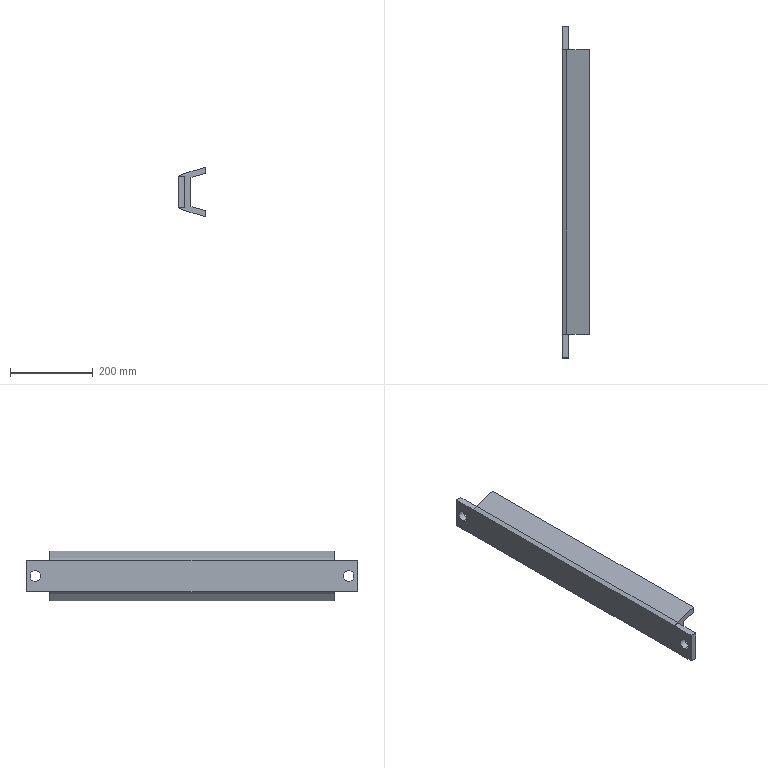Part | SolidWorks | features ICE 2, Extrusion 1, MirrorPattern 1 | 1 solid | 24 faces | box 65 x 800 x 120 mm | volume 2622134 mm3 | plane 20 | cylinder 4 | commonest cylinder face diameters 26 x4
STEP:
#1=CARTESIAN_POINT('',(15.,-377.5,-13.));
#2=VERTEX_POINT('',#1);
#3=CARTESIAN_POINT('',(15.,-377.5,13.));
#4=VERTEX_POINT('',#3);
#5=CARTESIAN_POINT('',(15.,-377.5,0.));
#6=DIRECTION('',(-1.,0.,0.));
#7=DIRECTION('',(0.,0.,1.));
#8=AXIS2_PLACEMENT_3D('',#5,#6,#7);
#9=CIRCLE('',#8,13.);
#10=EDGE_CURVE('',#2,#4,#9,.T.);
#11=ORIENTED_EDGE('',*,*,#10,.F.);
#12=CARTESIAN_POINT('',(0.,-377.5,-13.));
#13=VERTEX_POINT('',#12);
#14=CARTESIAN_POINT('',(57.5,-377.5,-13.));
#15=DIRECTION('',(-1.,0.,0.));
#16=VECTOR('',#15,1000.);
#17=LINE('',#14,#16);
#18=EDGE_CURVE('',#2,#13,#17,.T.);
#19=ORIENTED_EDGE('',*,*,#18,.T.);
#20=CARTESIAN_POINT('',(0.,-377.5,13.));
#21=VERTEX_POINT('',#20);
#22=CARTESIAN_POINT('',(0.,-377.5,0.));
#23=DIRECTION('',(-1.,0.,0.));
#24=DIRECTION('',(0.,0.,1.));
#25=AXIS2_PLACEMENT_3D('',#22,#23,#24);
#26=CIRCLE('',#25,13.);
#27=EDGE_CURVE('',#13,#21,#26,.T.);
#28=ORIENTED_EDGE('',*,*,#27,.T.);
#29=CARTESIAN_POINT('',(57.5,-377.5,13.));
#30=DIRECTION('',(-1.,0.,0.));
#31=VECTOR('',#30,1000.);
#32=LINE('',#29,#31);
#33=EDGE_CURVE('',#4,#21,#32,.T.);
#34=ORIENTED_EDGE('',*,*,#33,.F.);
#35=EDGE_LOOP('',(#11,#19,#28,#34));
#36=FACE_OUTER_BOUND('',#35,.T.);
#37=CARTESIAN_POINT('',(57.5,-377.5,0.));
#38=DIRECTION('',(-1.,0.,0.));
#39=DIRECTION('',(0.,0.,1.));
#40=AXIS2_PLACEMENT_3D('',#37,#38,#39);
#41=CYLINDRICAL_SURFACE('',#40,13.);
#42=ADVANCED_FACE('',(#36),#41,.F.);
#43=CARTESIAN_POINT('',(15.,377.5,13.));
#44=VERTEX_POINT('',#43);
#45=CARTESIAN_POINT('',(15.,377.5,-13.));
#46=VERTEX_POINT('',#45);
#47=CARTESIAN_POINT('',(15.,377.5,0.));
#48=DIRECTION('',(1.,0.,0.));
#49=DIRECTION('',(0.,0.,-1.));
#50=AXIS2_PLACEMENT_3D('',#47,#48,#49);
#51=CIRCLE('',#50,13.);
#52=EDGE_CURVE('',#44,#46,#51,.T.);
#53=ORIENTED_EDGE('',*,*,#52,.T.);
#54=CARTESIAN_POINT('',(0.,377.5,-13.));
#55=VERTEX_POINT('',#54);
#56=CARTESIAN_POINT('',(57.5,377.5,-13.));
#57=DIRECTION('',(-1.,0.,0.));
#58=VECTOR('',#57,1000.);
#59=LINE('',#56,#58);
#60=EDGE_CURVE('',#46,#55,#59,.T.);
#61=ORIENTED_EDGE('',*,*,#60,.T.);
#62=CARTESIAN_POINT('',(0.,377.5,13.));
#63=VERTEX_POINT('',#62);
#64=CARTESIAN_POINT('',(0.,377.5,0.));
#65=DIRECTION('',(-1.,0.,0.));
#66=DIRECTION('',(0.,0.,1.));
#67=AXIS2_PLACEMENT_3D('',#64,#65,#66);
#68=CIRCLE('',#67,13.);
#69=EDGE_CURVE('',#55,#63,#68,.T.);
#70=ORIENTED_EDGE('',*,*,#69,.T.);
#71=CARTESIAN_POINT('',(57.5,377.5,13.));
#72=DIRECTION('',(-1.,0.,0.));
#73=VECTOR('',#72,1000.);
#74=LINE('',#71,#73);
#75=EDGE_CURVE('',#44,#63,#74,.T.);
#76=ORIENTED_EDGE('',*,*,#75,.F.);
#77=EDGE_LOOP('',(#53,#61,#70,#76));
#78=FACE_OUTER_BOUND('',#77,.T.);
#79=CARTESIAN_POINT('',(57.5,377.5,0.));
#80=DIRECTION('',(-1.,0.,0.));
#81=DIRECTION('',(0.,0.,1.));
#82=AXIS2_PLACEMENT_3D('',#79,#80,#81);
#83=CYLINDRICAL_SURFACE('',#82,13.);
#84=ADVANCED_FACE('',(#78),#83,.F.);
#85=CARTESIAN_POINT('',(10.,342.5,-42.882));
#86=VERTEX_POINT('',#85);
#87=CARTESIAN_POINT('',(0.,342.5,-37.5));
#88=VERTEX_POINT('',#87);
#89=CARTESIAN_POINT('',(0.,342.5,-37.5));
#90=DIRECTION('',(-0.8806,0.,0.4739));
#91=VECTOR('',#90,1000.);
#92=LINE('',#89,#91);
#93=EDGE_CURVE('',#86,#88,#92,.T.);
#94=ORIENTED_EDGE('',*,*,#93,.T.);
#95=CARTESIAN_POINT('',(15.,342.5,-37.5));
#96=VERTEX_POINT('',#95);
#97=CARTESIAN_POINT('',(0.,342.5,-37.5));
#98=DIRECTION('',(1.,0.,0.));
#99=VECTOR('',#98,1000.);
#100=LINE('',#97,#99);
#101=EDGE_CURVE('',#88,#96,#100,.T.);
#102=ORIENTED_EDGE('',*,*,#101,.T.);
#103=CARTESIAN_POINT('',(15.,342.5,37.5));
#104=VERTEX_POINT('',#103);
#105=CARTESIAN_POINT('',(15.,342.5,37.5));
#106=DIRECTION('',(0.,0.,1.));
#107=VECTOR('',#106,1000.);
#108=LINE('',#105,#107);
#109=EDGE_CURVE('',#96,#104,#108,.T.);
#110=ORIENTED_EDGE('',*,*,#109,.T.);
#111=CARTESIAN_POINT('',(0.,342.5,37.5));
#112=VERTEX_POINT('',#111);
#113=CARTESIAN_POINT('',(0.,342.5,37.5));
#114=DIRECTION('',(-1.,0.,0.));
#115=VECTOR('',#114,1000.);
#116=LINE('',#113,#115);
#117=EDGE_CURVE('',#104,#112,#116,.T.);
#118=ORIENTED_EDGE('',*,*,#117,.T.);
#119=CARTESIAN_POINT('',(10.,342.5,42.882));
#120=VERTEX_POINT('',#119);
#121=CARTESIAN_POINT('',(0.,342.5,37.5));
#122=DIRECTION('',(0.8806,0.,0.4739));
#123=VECTOR('',#122,1000.);
#124=LINE('',#121,#123);
#125=EDGE_CURVE('',#112,#120,#124,.T.);
#126=ORIENTED_EDGE('',*,*,#125,.T.);
#127=CARTESIAN_POINT('',(65.,342.5,60.));
#128=VERTEX_POINT('',#127);
#129=CARTESIAN_POINT('',(10.,342.5,42.882));
#130=DIRECTION('',(0.9548,0.,0.2972));
#131=VECTOR('',#130,1000.);
#132=LINE('',#129,#131);
#133=EDGE_CURVE('',#120,#128,#132,.T.);
#134=ORIENTED_EDGE('',*,*,#133,.T.);
#135=CARTESIAN_POINT('',(65.,342.5,45.));
#136=VERTEX_POINT('',#135);
#137=CARTESIAN_POINT('',(65.,342.5,60.));
#138=DIRECTION('',(0.,0.,-1.));
#139=VECTOR('',#138,1000.);
#140=LINE('',#137,#139);
#141=EDGE_CURVE('',#128,#136,#140,.T.);
#142=ORIENTED_EDGE('',*,*,#141,.T.);
#143=CARTESIAN_POINT('',(30.,342.5,35.));
#144=VERTEX_POINT('',#143);
#145=CARTESIAN_POINT('',(65.,342.5,45.));
#146=DIRECTION('',(-0.9615,0.,-0.2747));
#147=VECTOR('',#146,1000.);
#148=LINE('',#145,#147);
#149=EDGE_CURVE('',#136,#144,#148,.T.);
#150=ORIENTED_EDGE('',*,*,#149,.T.);
#151=CARTESIAN_POINT('',(30.,342.5,-35.));
#152=VERTEX_POINT('',#151);
#153=CARTESIAN_POINT('',(30.,342.5,-35.));
#154=DIRECTION('',(0.,0.,-1.));
#155=VECTOR('',#154,1000.);
#156=LINE('',#153,#155);
#157=EDGE_CURVE('',#144,#152,#156,.T.);
#158=ORIENTED_EDGE('',*,*,#157,.T.);
#159=CARTESIAN_POINT('',(65.,342.5,-45.));
#160=VERTEX_POINT('',#159);
#161=CARTESIAN_POINT('',(65.,342.5,-45.));
#162=DIRECTION('',(0.9615,0.,-0.2747));
#163=VECTOR('',#162,1000.);
#164=LINE('',#161,#163);
#165=EDGE_CURVE('',#152,#160,#164,.T.);
#166=ORIENTED_EDGE('',*,*,#165,.T.);
#167=CARTESIAN_POINT('',(65.,342.5,-60.));
#168=VERTEX_POINT('',#167);
#169=CARTESIAN_POINT('',(65.,342.5,-60.));
#170=DIRECTION('',(0.,0.,-1.));
#171=VECTOR('',#170,1000.);
#172=LINE('',#169,#171);
#173=EDGE_CURVE('',#160,#168,#172,.T.);
#174=ORIENTED_EDGE('',*,*,#173,.T.);
#175=CARTESIAN_POINT('',(10.,342.5,-42.882));
#176=DIRECTION('',(-0.9548,0.,0.2972));
#177=VECTOR('',#176,1000.);
#178=LINE('',#175,#177);
#179=EDGE_CURVE('',#168,#86,#178,.T.);
#180=ORIENTED_EDGE('',*,*,#179,.T.);
#181=EDGE_LOOP('',(#94,#102,#110,#118,#126,#134,#142,#150,#158,#166,#174,#180));
#182=FACE_OUTER_BOUND('',#181,.T.);
#183=CARTESIAN_POINT('',(0.,342.5,0.));
#184=DIRECTION('',(0.,1.,0.));
#185=DIRECTION('',(0.,0.,1.));
#186=AXIS2_PLACEMENT_3D('',#183,#184,#185);
#187=PLANE('',#186);
#188=ADVANCED_FACE('',(#182),#187,.T.);
#189=CARTESIAN_POINT('',(15.,-342.5,37.5));
#190=VERTEX_POINT('',#189);
#191=CARTESIAN_POINT('',(0.,-342.5,37.5));
#192=VERTEX_POINT('',#191);
#193=CARTESIAN_POINT('',(0.,-342.5,37.5));
#194=DIRECTION('',(-1.,0.,0.));
#195=VECTOR('',#194,1000.);
#196=LINE('',#193,#195);
#197=EDGE_CURVE('',#190,#192,#196,.T.);
#198=ORIENTED_EDGE('',*,*,#197,.F.);
#199=CARTESIAN_POINT('',(15.,-342.5,-37.5));
#200=VERTEX_POINT('',#199);
#201=CARTESIAN_POINT('',(15.,-342.5,37.5));
#202=DIRECTION('',(0.,0.,1.));
#203=VECTOR('',#202,1000.);
#204=LINE('',#201,#203);
#205=EDGE_CURVE('',#200,#190,#204,.T.);
#206=ORIENTED_EDGE('',*,*,#205,.F.);
#207=CARTESIAN_POINT('',(0.,-342.5,-37.5));
#208=VERTEX_POINT('',#207);
#209=CARTESIAN_POINT('',(0.,-342.5,-37.5));
#210=DIRECTION('',(1.,0.,0.));
#211=VECTOR('',#210,1000.);
#212=LINE('',#209,#211);
#213=EDGE_CURVE('',#208,#200,#212,.T.);
#214=ORIENTED_EDGE('',*,*,#213,.F.);
#215=CARTESIAN_POINT('',(10.,-342.5,-42.882));
#216=VERTEX_POINT('',#215);
#217=CARTESIAN_POINT('',(0.,-342.5,-37.5));
#218=DIRECTION('',(-0.8806,0.,0.4739));
#219=VECTOR('',#218,1000.);
#220=LINE('',#217,#219);
#221=EDGE_CURVE('',#216,#208,#220,.T.);
#222=ORIENTED_EDGE('',*,*,#221,.F.);
#223=CARTESIAN_POINT('',(65.,-342.5,-60.));
#224=VERTEX_POINT('',#223);
#225=CARTESIAN_POINT('',(10.,-342.5,-42.882));
#226=DIRECTION('',(-0.9548,0.,0.2972));
#227=VECTOR('',#226,1000.);
#228=LINE('',#225,#227);
#229=EDGE_CURVE('',#224,#216,#228,.T.);
#230=ORIENTED_EDGE('',*,*,#229,.F.);
#231=CARTESIAN_POINT('',(65.,-342.5,-45.));
#232=VERTEX_POINT('',#231);
#233=CARTESIAN_POINT('',(65.,-342.5,-60.));
#234=DIRECTION('',(0.,0.,-1.));
#235=VECTOR('',#234,1000.);
#236=LINE('',#233,#235);
#237=EDGE_CURVE('',#232,#224,#236,.T.);
#238=ORIENTED_EDGE('',*,*,#237,.F.);
#239=CARTESIAN_POINT('',(30.,-342.5,-35.));
#240=VERTEX_POINT('',#239);
#241=CARTESIAN_POINT('',(65.,-342.5,-45.));
#242=DIRECTION('',(0.9615,0.,-0.2747));
#243=VECTOR('',#242,1000.);
#244=LINE('',#241,#243);
#245=EDGE_CURVE('',#240,#232,#244,.T.);
#246=ORIENTED_EDGE('',*,*,#245,.F.);
#247=CARTESIAN_POINT('',(30.,-342.5,35.));
#248=VERTEX_POINT('',#247);
#249=CARTESIAN_POINT('',(30.,-342.5,-35.));
#250=DIRECTION('',(0.,0.,-1.));
#251=VECTOR('',#250,1000.);
#252=LINE('',#249,#251);
#253=EDGE_CURVE('',#248,#240,#252,.T.);
#254=ORIENTED_EDGE('',*,*,#253,.F.);
#255=CARTESIAN_POINT('',(65.,-342.5,45.));
#256=VERTEX_POINT('',#255);
#257=CARTESIAN_POINT('',(65.,-342.5,45.));
#258=DIRECTION('',(-0.9615,0.,-0.2747));
#259=VECTOR('',#258,1000.);
#260=LINE('',#257,#259);
#261=EDGE_CURVE('',#256,#248,#260,.T.);
#262=ORIENTED_EDGE('',*,*,#261,.F.);
#263=CARTESIAN_POINT('',(65.,-342.5,60.));
#264=VERTEX_POINT('',#263);
#265=CARTESIAN_POINT('',(65.,-342.5,60.));
#266=DIRECTION('',(0.,0.,-1.));
#267=VECTOR('',#266,1000.);
#268=LINE('',#265,#267);
#269=EDGE_CURVE('',#264,#256,#268,.T.);
#270=ORIENTED_EDGE('',*,*,#269,.F.);
#271=CARTESIAN_POINT('',(10.,-342.5,42.882));
#272=VERTEX_POINT('',#271);
#273=CARTESIAN_POINT('',(10.,-342.5,42.882));
#274=DIRECTION('',(0.9548,0.,0.2972));
#275=VECTOR('',#274,1000.);
#276=LINE('',#273,#275);
#277=EDGE_CURVE('',#272,#264,#276,.T.);
#278=ORIENTED_EDGE('',*,*,#277,.F.);
#279=CARTESIAN_POINT('',(0.,-342.5,37.5));
#280=DIRECTION('',(0.8806,0.,0.4739));
#281=VECTOR('',#280,1000.);
#282=LINE('',#279,#281);
#283=EDGE_CURVE('',#192,#272,#282,.T.);
#284=ORIENTED_EDGE('',*,*,#283,.F.);
#285=EDGE_LOOP('',(#198,#206,#214,#222,#230,#238,#246,#254,#262,#270,#278,#284));
#286=FACE_OUTER_BOUND('',#285,.T.);
#287=CARTESIAN_POINT('',(0.,-342.5,0.));
#288=DIRECTION('',(0.,1.,0.));
#289=DIRECTION('',(0.,0.,1.));
#290=AXIS2_PLACEMENT_3D('',#287,#288,#289);
#291=PLANE('',#290);
#292=ADVANCED_FACE('',(#286),#291,.F.);
#293=ORIENTED_EDGE('',*,*,#261,.T.);
#294=CARTESIAN_POINT('',(30.,342.5,35.));
#295=DIRECTION('',(0.,-1.,0.));
#296=VECTOR('',#295,1000.);
#297=LINE('',#294,#296);
#298=EDGE_CURVE('',#144,#248,#297,.T.);
#299=ORIENTED_EDGE('',*,*,#298,.F.);
#300=ORIENTED_EDGE('',*,*,#149,.F.);
#301=CARTESIAN_POINT('',(65.,342.5,45.));
#302=DIRECTION('',(0.,-1.,0.));
#303=VECTOR('',#302,1000.);
#304=LINE('',#301,#303);
#305=EDGE_CURVE('',#136,#256,#304,.T.);
#306=ORIENTED_EDGE('',*,*,#305,.T.);
#307=EDGE_LOOP('',(#293,#299,#300,#306));
#308=FACE_OUTER_BOUND('',#307,.T.);
#309=CARTESIAN_POINT('',(65.,342.5,45.));
#310=DIRECTION('',(-0.2747,0.,0.9615));
#311=DIRECTION('',(0.9615,0.,0.2747));
#312=AXIS2_PLACEMENT_3D('',#309,#310,#311);
#313=PLANE('',#312);
#314=ADVANCED_FACE('',(#308),#313,.F.);
#315=ORIENTED_EDGE('',*,*,#253,.T.);
#316=CARTESIAN_POINT('',(30.,342.5,-35.));
#317=DIRECTION('',(0.,-1.,0.));
#318=VECTOR('',#317,1000.);
#319=LINE('',#316,#318);
#320=EDGE_CURVE('',#152,#240,#319,.T.);
#321=ORIENTED_EDGE('',*,*,#320,.F.);
#322=ORIENTED_EDGE('',*,*,#157,.F.);
#323=ORIENTED_EDGE('',*,*,#298,.T.);
#324=EDGE_LOOP('',(#315,#321,#322,#323));
#325=FACE_OUTER_BOUND('',#324,.T.);
#326=CARTESIAN_POINT('',(30.,342.5,-35.));
#327=DIRECTION('',(-1.,0.,0.));
#328=DIRECTION('',(0.,0.,1.));
#329=AXIS2_PLACEMENT_3D('',#326,#327,#328);
#330=PLANE('',#329);
#331=ADVANCED_FACE('',(#325),#330,.F.);
#332=ORIENTED_EDGE('',*,*,#245,.T.);
#333=CARTESIAN_POINT('',(65.,342.5,-45.));
#334=DIRECTION('',(0.,-1.,0.));
#335=VECTOR('',#334,1000.);
#336=LINE('',#333,#335);
#337=EDGE_CURVE('',#160,#232,#336,.T.);
#338=ORIENTED_EDGE('',*,*,#337,.F.);
#339=ORIENTED_EDGE('',*,*,#165,.F.);
#340=ORIENTED_EDGE('',*,*,#320,.T.);
#341=EDGE_LOOP('',(#332,#338,#339,#340));
#342=FACE_OUTER_BOUND('',#341,.T.);
#343=CARTESIAN_POINT('',(65.,342.5,-45.));
#344=DIRECTION('',(-0.2747,0.,-0.9615));
#345=DIRECTION('',(-0.9615,0.,0.2747));
#346=AXIS2_PLACEMENT_3D('',#343,#344,#345);
#347=PLANE('',#346);
#348=ADVANCED_FACE('',(#342),#347,.F.);
#349=ORIENTED_EDGE('',*,*,#237,.T.);
#350=CARTESIAN_POINT('',(65.,342.5,-60.));
#351=DIRECTION('',(0.,-1.,0.));
#352=VECTOR('',#351,1000.);
#353=LINE('',#350,#352);
#354=EDGE_CURVE('',#168,#224,#353,.T.);
#355=ORIENTED_EDGE('',*,*,#354,.F.);
#356=ORIENTED_EDGE('',*,*,#173,.F.);
#357=ORIENTED_EDGE('',*,*,#337,.T.);
#358=EDGE_LOOP('',(#349,#355,#356,#357));
#359=FACE_OUTER_BOUND('',#358,.T.);
#360=CARTESIAN_POINT('',(65.,342.5,-60.));
#361=DIRECTION('',(-1.,0.,0.));
#362=DIRECTION('',(0.,0.,1.));
#363=AXIS2_PLACEMENT_3D('',#360,#361,#362);
#364=PLANE('',#363);
#365=ADVANCED_FACE('',(#359),#364,.F.);
#366=ORIENTED_EDGE('',*,*,#229,.T.);
#367=CARTESIAN_POINT('',(10.,342.5,-42.882));
#368=DIRECTION('',(0.,-1.,0.));
#369=VECTOR('',#368,1000.);
#370=LINE('',#367,#369);
#371=EDGE_CURVE('',#86,#216,#370,.T.);
#372=ORIENTED_EDGE('',*,*,#371,.F.);
#373=ORIENTED_EDGE('',*,*,#179,.F.);
#374=ORIENTED_EDGE('',*,*,#354,.T.);
#375=EDGE_LOOP('',(#366,#372,#373,#374));
#376=FACE_OUTER_BOUND('',#375,.T.);
#377=CARTESIAN_POINT('',(10.,342.5,-42.882));
#378=DIRECTION('',(0.2972,0.,0.9548));
#379=DIRECTION('',(0.9548,0.,-0.2972));
#380=AXIS2_PLACEMENT_3D('',#377,#378,#379);
#381=PLANE('',#380);
#382=ADVANCED_FACE('',(#376),#381,.F.);
#383=ORIENTED_EDGE('',*,*,#221,.T.);
#384=CARTESIAN_POINT('',(0.,342.5,-37.5));
#385=DIRECTION('',(0.,-1.,0.));
#386=VECTOR('',#385,1000.);
#387=LINE('',#384,#386);
#388=EDGE_CURVE('',#88,#208,#387,.T.);
#389=ORIENTED_EDGE('',*,*,#388,.F.);
#390=ORIENTED_EDGE('',*,*,#93,.F.);
#391=ORIENTED_EDGE('',*,*,#371,.T.);
#392=EDGE_LOOP('',(#383,#389,#390,#391));
#393=FACE_OUTER_BOUND('',#392,.T.);
#394=CARTESIAN_POINT('',(0.,342.5,-37.5));
#395=DIRECTION('',(0.4739,0.,0.8806));
#396=DIRECTION('',(0.8806,0.,-0.4739));
#397=AXIS2_PLACEMENT_3D('',#394,#395,#396);
#398=PLANE('',#397);
#399=ADVANCED_FACE('',(#393),#398,.F.);
#400=CARTESIAN_POINT('',(0.,-377.5,0.));
#401=DIRECTION('',(-1.,0.,0.));
#402=DIRECTION('',(0.,0.,1.));
#403=AXIS2_PLACEMENT_3D('',#400,#401,#402);
#404=CIRCLE('',#403,13.);
#405=EDGE_CURVE('',#21,#13,#404,.T.);
#406=ORIENTED_EDGE('',*,*,#405,.F.);
#407=ORIENTED_EDGE('',*,*,#27,.F.);
#408=EDGE_LOOP('',(#406,#407));
#409=FACE_BOUND('',#408,.T.);
#410=CARTESIAN_POINT('',(0.,377.5,0.));
#411=DIRECTION('',(-1.,0.,0.));
#412=DIRECTION('',(0.,0.,1.));
#413=AXIS2_PLACEMENT_3D('',#410,#411,#412);
#414=CIRCLE('',#413,13.);
#415=EDGE_CURVE('',#63,#55,#414,.T.);
#416=ORIENTED_EDGE('',*,*,#415,.F.);
#417=ORIENTED_EDGE('',*,*,#69,.F.);
#418=EDGE_LOOP('',(#416,#417));
#419=FACE_BOUND('',#418,.T.);
#420=ORIENTED_EDGE('',*,*,#388,.T.);
#421=CARTESIAN_POINT('',(0.,-400.,-37.5));
#422=VERTEX_POINT('',#421);
#423=CARTESIAN_POINT('',(0.,-400.,-37.5));
#424=DIRECTION('',(0.,1.,0.));
#425=VECTOR('',#424,1000.);
#426=LINE('',#423,#425);
#427=EDGE_CURVE('',#422,#208,#426,.T.);
#428=ORIENTED_EDGE('',*,*,#427,.F.);
#429=CARTESIAN_POINT('',(0.,-400.,37.5));
#430=VERTEX_POINT('',#429);
#431=CARTESIAN_POINT('',(0.,-400.,37.5));
#432=DIRECTION('',(0.,0.,-1.));
#433=VECTOR('',#432,1000.);
#434=LINE('',#431,#433);
#435=EDGE_CURVE('',#430,#422,#434,.T.);
#436=ORIENTED_EDGE('',*,*,#435,.F.);
#437=CARTESIAN_POINT('',(0.,-400.,37.5));
#438=DIRECTION('',(0.,1.,0.));
#439=VECTOR('',#438,1000.);
#440=LINE('',#437,#439);
#441=EDGE_CURVE('',#430,#192,#440,.T.);
#442=ORIENTED_EDGE('',*,*,#441,.T.);
#443=CARTESIAN_POINT('',(0.,342.5,37.5));
#444=DIRECTION('',(0.,-1.,0.));
#445=VECTOR('',#444,1000.);
#446=LINE('',#443,#445);
#447=EDGE_CURVE('',#112,#192,#446,.T.);
#448=ORIENTED_EDGE('',*,*,#447,.F.);
#449=CARTESIAN_POINT('',(0.,400.,37.5));
#450=VERTEX_POINT('',#449);
#451=CARTESIAN_POINT('',(0.,400.,37.5));
#452=DIRECTION('',(0.,-1.,0.));
#453=VECTOR('',#452,1000.);
#454=LINE('',#451,#453);
#455=EDGE_CURVE('',#450,#112,#454,.T.);
#456=ORIENTED_EDGE('',*,*,#455,.F.);
#457=CARTESIAN_POINT('',(0.,400.,-37.5));
#458=VERTEX_POINT('',#457);
#459=CARTESIAN_POINT('',(0.,400.,37.5));
#460=DIRECTION('',(0.,0.,-1.));
#461=VECTOR('',#460,1000.);
#462=LINE('',#459,#461);
#463=EDGE_CURVE('',#450,#458,#462,.T.);
#464=ORIENTED_EDGE('',*,*,#463,.T.);
#465=CARTESIAN_POINT('',(0.,400.,-37.5));
#466=DIRECTION('',(0.,-1.,0.));
#467=VECTOR('',#466,1000.);
#468=LINE('',#465,#467);
#469=EDGE_CURVE('',#458,#88,#468,.T.);
#470=ORIENTED_EDGE('',*,*,#469,.T.);
#471=EDGE_LOOP('',(#420,#428,#436,#442,#448,#456,#464,#470));
#472=FACE_OUTER_BOUND('',#471,.T.);
#473=CARTESIAN_POINT('',(0.,342.5,37.5));
#474=DIRECTION('',(1.,0.,0.));
#475=DIRECTION('',(0.,0.,-1.));
#476=AXIS2_PLACEMENT_3D('',#473,#474,#475);
#477=PLANE('',#476);
#478=ADVANCED_FACE('',(#409,#419,#472),#477,.F.);
#479=ORIENTED_EDGE('',*,*,#283,.T.);
#480=CARTESIAN_POINT('',(10.,342.5,42.882));
#481=DIRECTION('',(0.,-1.,0.));
#482=VECTOR('',#481,1000.);
#483=LINE('',#480,#482);
#484=EDGE_CURVE('',#120,#272,#483,.T.);
#485=ORIENTED_EDGE('',*,*,#484,.F.);
#486=ORIENTED_EDGE('',*,*,#125,.F.);
#487=ORIENTED_EDGE('',*,*,#447,.T.);
#488=EDGE_LOOP('',(#479,#485,#486,#487));
#489=FACE_OUTER_BOUND('',#488,.T.);
#490=CARTESIAN_POINT('',(0.,342.5,37.5));
#491=DIRECTION('',(0.4739,0.,-0.8806));
#492=DIRECTION('',(-0.8806,0.,-0.4739));
#493=AXIS2_PLACEMENT_3D('',#490,#491,#492);
#494=PLANE('',#493);
#495=ADVANCED_FACE('',(#489),#494,.F.);
#496=ORIENTED_EDGE('',*,*,#277,.T.);
#497=CARTESIAN_POINT('',(65.,342.5,60.));
#498=DIRECTION('',(0.,-1.,0.));
#499=VECTOR('',#498,1000.);
#500=LINE('',#497,#499);
#501=EDGE_CURVE('',#128,#264,#500,.T.);
#502=ORIENTED_EDGE('',*,*,#501,.F.);
#503=ORIENTED_EDGE('',*,*,#133,.F.);
#504=ORIENTED_EDGE('',*,*,#484,.T.);
#505=EDGE_LOOP('',(#496,#502,#503,#504));
#506=FACE_OUTER_BOUND('',#505,.T.);
#507=CARTESIAN_POINT('',(10.,342.5,42.882));
#508=DIRECTION('',(0.2972,0.,-0.9548));
#509=DIRECTION('',(-0.9548,0.,-0.2972));
#510=AXIS2_PLACEMENT_3D('',#507,#508,#509);
#511=PLANE('',#510);
#512=ADVANCED_FACE('',(#506),#511,.F.);
#513=ORIENTED_EDGE('',*,*,#269,.T.);
#514=ORIENTED_EDGE('',*,*,#305,.F.);
#515=ORIENTED_EDGE('',*,*,#141,.F.);
#516=ORIENTED_EDGE('',*,*,#501,.T.);
#517=EDGE_LOOP('',(#513,#514,#515,#516));
#518=FACE_OUTER_BOUND('',#517,.T.);
#519=CARTESIAN_POINT('',(65.,342.5,60.));
#520=DIRECTION('',(-1.,0.,0.));
#521=DIRECTION('',(0.,0.,1.));
#522=AXIS2_PLACEMENT_3D('',#519,#520,#521);
#523=PLANE('',#522);
#524=ADVANCED_FACE('',(#518),#523,.F.);
#525=ORIENTED_EDGE('',*,*,#213,.T.);
#526=CARTESIAN_POINT('',(15.,-400.,-37.5));
#527=VERTEX_POINT('',#526);
#528=CARTESIAN_POINT('',(15.,-400.,-37.5));
#529=DIRECTION('',(0.,1.,0.));
#530=VECTOR('',#529,1000.);
#531=LINE('',#528,#530);
#532=EDGE_CURVE('',#527,#200,#531,.T.);
#533=ORIENTED_EDGE('',*,*,#532,.F.);
#534=CARTESIAN_POINT('',(0.,-400.,-37.5));
#535=DIRECTION('',(1.,0.,0.));
#536=VECTOR('',#535,1000.);
#537=LINE('',#534,#536);
#538=EDGE_CURVE('',#422,#527,#537,.T.);
#539=ORIENTED_EDGE('',*,*,#538,.F.);
#540=ORIENTED_EDGE('',*,*,#427,.T.);
#541=EDGE_LOOP('',(#525,#533,#539,#540));
#542=FACE_OUTER_BOUND('',#541,.T.);
#543=CARTESIAN_POINT('',(0.,-400.,-37.5));
#544=DIRECTION('',(0.,0.,1.));
#545=DIRECTION('',(1.,0.,0.));
#546=AXIS2_PLACEMENT_3D('',#543,#544,#545);
#547=PLANE('',#546);
#548=ADVANCED_FACE('',(#542),#547,.F.);
#549=CARTESIAN_POINT('',(15.,-377.5,0.));
#550=DIRECTION('',(-1.,0.,0.));
#551=DIRECTION('',(0.,0.,1.));
#552=AXIS2_PLACEMENT_3D('',#549,#550,#551);
#553=CIRCLE('',#552,13.);
#554=EDGE_CURVE('',#4,#2,#553,.T.);
#555=ORIENTED_EDGE('',*,*,#554,.T.);
#556=ORIENTED_EDGE('',*,*,#10,.T.);
#557=EDGE_LOOP('',(#555,#556));
#558=FACE_BOUND('',#557,.T.);
#559=ORIENTED_EDGE('',*,*,#205,.T.);
#560=CARTESIAN_POINT('',(15.,-400.,37.5));
#561=VERTEX_POINT('',#560);
#562=CARTESIAN_POINT('',(15.,-400.,37.5));
#563=DIRECTION('',(0.,1.,0.));
#564=VECTOR('',#563,1000.);
#565=LINE('',#562,#564);
#566=EDGE_CURVE('',#561,#190,#565,.T.);
#567=ORIENTED_EDGE('',*,*,#566,.F.);
#568=CARTESIAN_POINT('',(15.,-400.,37.5));
#569=DIRECTION('',(0.,0.,1.));
#570=VECTOR('',#569,1000.);
#571=LINE('',#568,#570);
#572=EDGE_CURVE('',#527,#561,#571,.T.);
#573=ORIENTED_EDGE('',*,*,#572,.F.);
#574=ORIENTED_EDGE('',*,*,#532,.T.);
#575=EDGE_LOOP('',(#559,#567,#573,#574));
#576=FACE_OUTER_BOUND('',#575,.T.);
#577=CARTESIAN_POINT('',(15.,-400.,37.5));
#578=DIRECTION('',(-1.,0.,0.));
#579=DIRECTION('',(0.,0.,1.));
#580=AXIS2_PLACEMENT_3D('',#577,#578,#579);
#581=PLANE('',#580);
#582=ADVANCED_FACE('',(#558,#576),#581,.F.);
#583=ORIENTED_EDGE('',*,*,#197,.T.);
#584=ORIENTED_EDGE('',*,*,#441,.F.);
#585=CARTESIAN_POINT('',(0.,-400.,37.5));
#586=DIRECTION('',(-1.,0.,0.));
#587=VECTOR('',#586,1000.);
#588=LINE('',#585,#587);
#589=EDGE_CURVE('',#561,#430,#588,.T.);
#590=ORIENTED_EDGE('',*,*,#589,.F.);
#591=ORIENTED_EDGE('',*,*,#566,.T.);
#592=EDGE_LOOP('',(#583,#584,#590,#591));
#593=FACE_OUTER_BOUND('',#592,.T.);
#594=CARTESIAN_POINT('',(0.,-400.,37.5));
#595=DIRECTION('',(0.,0.,-1.));
#596=DIRECTION('',(-1.,0.,0.));
#597=AXIS2_PLACEMENT_3D('',#594,#595,#596);
#598=PLANE('',#597);
#599=ADVANCED_FACE('',(#593),#598,.F.);
#600=ORIENTED_EDGE('',*,*,#435,.T.);
#601=ORIENTED_EDGE('',*,*,#538,.T.);
#602=ORIENTED_EDGE('',*,*,#572,.T.);
#603=ORIENTED_EDGE('',*,*,#589,.T.);
#604=EDGE_LOOP('',(#600,#601,#602,#603));
#605=FACE_OUTER_BOUND('',#604,.T.);
#606=CARTESIAN_POINT('',(0.,-400.,0.));
#607=DIRECTION('',(0.,-1.,0.));
#608=DIRECTION('',(0.,0.,-1.));
#609=AXIS2_PLACEMENT_3D('',#606,#607,#608);
#610=PLANE('',#609);
#611=ADVANCED_FACE('',(#605),#610,.T.);
#612=ORIENTED_EDGE('',*,*,#117,.F.);
#613=CARTESIAN_POINT('',(15.,400.,37.5));
#614=VERTEX_POINT('',#613);
#615=CARTESIAN_POINT('',(15.,400.,37.5));
#616=DIRECTION('',(0.,-1.,0.));
#617=VECTOR('',#616,1000.);
#618=LINE('',#615,#617);
#619=EDGE_CURVE('',#614,#104,#618,.T.);
#620=ORIENTED_EDGE('',*,*,#619,.F.);
#621=CARTESIAN_POINT('',(0.,400.,37.5));
#622=DIRECTION('',(-1.,0.,0.));
#623=VECTOR('',#622,1000.);
#624=LINE('',#621,#623);
#625=EDGE_CURVE('',#614,#450,#624,.T.);
#626=ORIENTED_EDGE('',*,*,#625,.T.);
#627=ORIENTED_EDGE('',*,*,#455,.T.);
#628=EDGE_LOOP('',(#612,#620,#626,#627));
#629=FACE_OUTER_BOUND('',#628,.T.);
#630=CARTESIAN_POINT('',(0.,400.,37.5));
#631=DIRECTION('',(0.,0.,1.));
#632=DIRECTION('',(1.,0.,0.));
#633=AXIS2_PLACEMENT_3D('',#630,#631,#632);
#634=PLANE('',#633);
#635=ADVANCED_FACE('',(#629),#634,.T.);
#636=ORIENTED_EDGE('',*,*,#52,.F.);
#637=CARTESIAN_POINT('',(15.,377.5,0.));
#638=DIRECTION('',(1.,0.,0.));
#639=DIRECTION('',(0.,0.,-1.));
#640=AXIS2_PLACEMENT_3D('',#637,#638,#639);
#641=CIRCLE('',#640,13.);
#642=EDGE_CURVE('',#46,#44,#641,.T.);
#643=ORIENTED_EDGE('',*,*,#642,.F.);
#644=EDGE_LOOP('',(#636,#643));
#645=FACE_BOUND('',#644,.T.);
#646=ORIENTED_EDGE('',*,*,#109,.F.);
#647=CARTESIAN_POINT('',(15.,400.,-37.5));
#648=VERTEX_POINT('',#647);
#649=CARTESIAN_POINT('',(15.,400.,-37.5));
#650=DIRECTION('',(0.,-1.,0.));
#651=VECTOR('',#650,1000.);
#652=LINE('',#649,#651);
#653=EDGE_CURVE('',#648,#96,#652,.T.);
#654=ORIENTED_EDGE('',*,*,#653,.F.);
#655=CARTESIAN_POINT('',(15.,400.,37.5));
#656=DIRECTION('',(0.,0.,1.));
#657=VECTOR('',#656,1000.);
#658=LINE('',#655,#657);
#659=EDGE_CURVE('',#648,#614,#658,.T.);
#660=ORIENTED_EDGE('',*,*,#659,.T.);
#661=ORIENTED_EDGE('',*,*,#619,.T.);
#662=EDGE_LOOP('',(#646,#654,#660,#661));
#663=FACE_OUTER_BOUND('',#662,.T.);
#664=CARTESIAN_POINT('',(15.,400.,37.5));
#665=DIRECTION('',(1.,0.,0.));
#666=DIRECTION('',(0.,0.,-1.));
#667=AXIS2_PLACEMENT_3D('',#664,#665,#666);
#668=PLANE('',#667);
#669=ADVANCED_FACE('',(#645,#663),#668,.T.);
#670=ORIENTED_EDGE('',*,*,#101,.F.);
#671=ORIENTED_EDGE('',*,*,#469,.F.);
#672=CARTESIAN_POINT('',(0.,400.,-37.5));
#673=DIRECTION('',(1.,0.,0.));
#674=VECTOR('',#673,1000.);
#675=LINE('',#672,#674);
#676=EDGE_CURVE('',#458,#648,#675,.T.);
#677=ORIENTED_EDGE('',*,*,#676,.T.);
#678=ORIENTED_EDGE('',*,*,#653,.T.);
#679=EDGE_LOOP('',(#670,#671,#677,#678));
#680=FACE_OUTER_BOUND('',#679,.T.);
#681=CARTESIAN_POINT('',(0.,400.,-37.5));
#682=DIRECTION('',(0.,0.,-1.));
#683=DIRECTION('',(-1.,0.,0.));
#684=AXIS2_PLACEMENT_3D('',#681,#682,#683);
#685=PLANE('',#684);
#686=ADVANCED_FACE('',(#680),#685,.T.);
#687=ORIENTED_EDGE('',*,*,#463,.F.);
#688=ORIENTED_EDGE('',*,*,#625,.F.);
#689=ORIENTED_EDGE('',*,*,#659,.F.);
#690=ORIENTED_EDGE('',*,*,#676,.F.);
#691=EDGE_LOOP('',(#687,#688,#689,#690));
#692=FACE_OUTER_BOUND('',#691,.T.);
#693=CARTESIAN_POINT('',(0.,400.,0.));
#694=DIRECTION('',(0.,1.,0.));
#695=DIRECTION('',(0.,0.,-1.));
#696=AXIS2_PLACEMENT_3D('',#693,#694,#695);
#697=PLANE('',#696);
#698=ADVANCED_FACE('',(#692),#697,.T.);
#699=ORIENTED_EDGE('',*,*,#60,.F.);
#700=ORIENTED_EDGE('',*,*,#642,.T.);
#701=ORIENTED_EDGE('',*,*,#75,.T.);
#702=ORIENTED_EDGE('',*,*,#415,.T.);
#703=EDGE_LOOP('',(#699,#700,#701,#702));
#704=FACE_OUTER_BOUND('',#703,.T.);
#705=CARTESIAN_POINT('',(57.5,377.5,0.));
#706=DIRECTION('',(-1.,0.,0.));
#707=DIRECTION('',(0.,0.,1.));
#708=AXIS2_PLACEMENT_3D('',#705,#706,#707);
#709=CYLINDRICAL_SURFACE('',#708,13.);
#710=ADVANCED_FACE('',(#704),#709,.F.);
#711=ORIENTED_EDGE('',*,*,#18,.F.);
#712=ORIENTED_EDGE('',*,*,#554,.F.);
#713=ORIENTED_EDGE('',*,*,#33,.T.);
#714=ORIENTED_EDGE('',*,*,#405,.T.);
#715=EDGE_LOOP('',(#711,#712,#713,#714));
#716=FACE_OUTER_BOUND('',#715,.T.);
#717=CARTESIAN_POINT('',(57.5,-377.5,0.));
#718=DIRECTION('',(-1.,0.,0.));
#719=DIRECTION('',(0.,0.,1.));
#720=AXIS2_PLACEMENT_3D('',#717,#718,#719);
#721=CYLINDRICAL_SURFACE('',#720,13.);
#722=ADVANCED_FACE('',(#716),#721,.F.);
#723=CLOSED_SHELL('',(#42,#84,#188,#292,#314,#331,#348,#365,#382,#399,#478,#495,#512,#524,#548,#582,#599,#611,#635,#669,#686,#698,#710,#722));
#724=MANIFOLD_SOLID_BREP('',#723);
#725=CARTESIAN_POINT('',(0.,0.,0.));
#726=DIRECTION('',(0.,0.,1.));
#727=DIRECTION('',(1.,0.,0.));
#728=AXIS2_PLACEMENT_3D('',#725,#726,#727);
#729=(LENGTH_UNIT()NAMED_UNIT(*)SI_UNIT(.MILLI.,.METRE.));
#730=UNCERTAINTY_MEASURE_WITH_UNIT(LENGTH_MEASURE(0.00001),#729,'','');
#731=(NAMED_UNIT(*)PLANE_ANGLE_UNIT()SI_UNIT($,.RADIAN.));
#732=(NAMED_UNIT(*)SI_UNIT($,.STERADIAN.)SOLID_ANGLE_UNIT());
#733=(GEOMETRIC_REPRESENTATION_CONTEXT(3)GLOBAL_UNCERTAINTY_ASSIGNED_CONTEXT((#730))GLOBAL_UNIT_ASSIGNED_CONTEXT((#729,#731,#732))REPRESENTATION_CONTEXT('',''));
#734=ADVANCED_BREP_SHAPE_REPRESENTATION('',(#724,#728),#733);